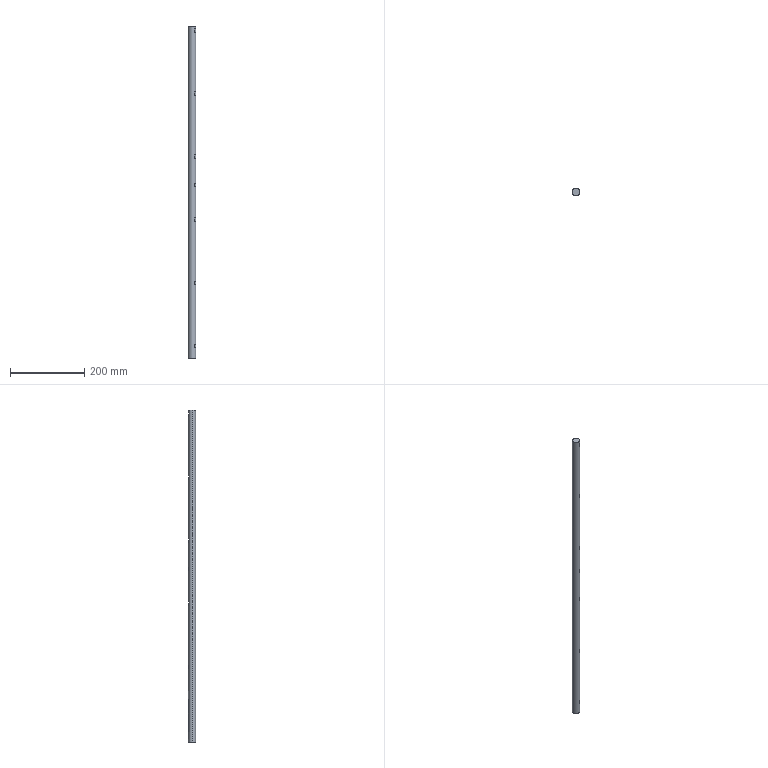Part | SolidWorks | features BaseBody 1 | 1 solid | 46 faces | box 20 x 20 x 895 mm | volume 280350 mm3 | plane 44 | cylinder 2 | commonest cylinder face diameters 20 x2
STEP:
#1=CARTESIAN_POINT('',(4.359,9.,877.5));
#2=VERTEX_POINT('',#1);
#3=CARTESIAN_POINT('',(-4.359,9.,877.5));
#4=VERTEX_POINT('',#3);
#5=CARTESIAN_POINT('',(0.,0.,877.5));
#6=DIRECTION('',(0.,0.,1.));
#7=DIRECTION('',(1.,0.,0.));
#8=AXIS2_PLACEMENT_3D('',#5,#6,#7);
#9=CIRCLE('',#8,10.);
#10=EDGE_CURVE('',#2,#4,#9,.T.);
#11=ORIENTED_EDGE('',*,*,#10,.F.);
#12=CARTESIAN_POINT('',(4.359,9.,887.5));
#13=VERTEX_POINT('',#12);
#14=CARTESIAN_POINT('',(4.359,9.,895.));
#15=DIRECTION('',(0.,0.,1.));
#16=VECTOR('',#15,1000.);
#17=LINE('',#14,#16);
#18=EDGE_CURVE('',#2,#13,#17,.T.);
#19=ORIENTED_EDGE('',*,*,#18,.T.);
#20=CARTESIAN_POINT('',(-4.359,9.,887.5));
#21=VERTEX_POINT('',#20);
#22=CARTESIAN_POINT('',(0.,0.,887.5));
#23=DIRECTION('',(0.,0.,1.));
#24=DIRECTION('',(1.,0.,0.));
#25=AXIS2_PLACEMENT_3D('',#22,#23,#24);
#26=CIRCLE('',#25,10.);
#27=EDGE_CURVE('',#13,#21,#26,.T.);
#28=ORIENTED_EDGE('',*,*,#27,.T.);
#29=CARTESIAN_POINT('',(-4.359,9.,895.));
#30=DIRECTION('',(0.,0.,-1.));
#31=VECTOR('',#30,1000.);
#32=LINE('',#29,#31);
#33=EDGE_CURVE('',#21,#4,#32,.T.);
#34=ORIENTED_EDGE('',*,*,#33,.T.);
#35=EDGE_LOOP('',(#11,#19,#28,#34));
#36=FACE_BOUND('',#35,.T.);
#37=CARTESIAN_POINT('',(4.359,9.,707.5));
#38=VERTEX_POINT('',#37);
#39=CARTESIAN_POINT('',(-4.359,9.,707.5));
#40=VERTEX_POINT('',#39);
#41=CARTESIAN_POINT('',(0.,0.,707.5));
#42=DIRECTION('',(0.,0.,1.));
#43=DIRECTION('',(1.,0.,0.));
#44=AXIS2_PLACEMENT_3D('',#41,#42,#43);
#45=CIRCLE('',#44,10.);
#46=EDGE_CURVE('',#38,#40,#45,.T.);
#47=ORIENTED_EDGE('',*,*,#46,.F.);
#48=CARTESIAN_POINT('',(4.359,9.,717.5));
#49=VERTEX_POINT('',#48);
#50=CARTESIAN_POINT('',(4.359,9.,895.));
#51=DIRECTION('',(0.,0.,1.));
#52=VECTOR('',#51,1000.);
#53=LINE('',#50,#52);
#54=EDGE_CURVE('',#38,#49,#53,.T.);
#55=ORIENTED_EDGE('',*,*,#54,.T.);
#56=CARTESIAN_POINT('',(-4.359,9.,717.5));
#57=VERTEX_POINT('',#56);
#58=CARTESIAN_POINT('',(0.,0.,717.5));
#59=DIRECTION('',(0.,0.,1.));
#60=DIRECTION('',(1.,0.,0.));
#61=AXIS2_PLACEMENT_3D('',#58,#59,#60);
#62=CIRCLE('',#61,10.);
#63=EDGE_CURVE('',#49,#57,#62,.T.);
#64=ORIENTED_EDGE('',*,*,#63,.T.);
#65=CARTESIAN_POINT('',(-4.359,9.,895.));
#66=DIRECTION('',(0.,0.,-1.));
#67=VECTOR('',#66,1000.);
#68=LINE('',#65,#67);
#69=EDGE_CURVE('',#57,#40,#68,.T.);
#70=ORIENTED_EDGE('',*,*,#69,.T.);
#71=EDGE_LOOP('',(#47,#55,#64,#70));
#72=FACE_BOUND('',#71,.T.);
#73=CARTESIAN_POINT('',(4.359,9.,537.5));
#74=VERTEX_POINT('',#73);
#75=CARTESIAN_POINT('',(-4.359,9.,537.5));
#76=VERTEX_POINT('',#75);
#77=CARTESIAN_POINT('',(0.,0.,537.5));
#78=DIRECTION('',(0.,0.,1.));
#79=DIRECTION('',(1.,0.,0.));
#80=AXIS2_PLACEMENT_3D('',#77,#78,#79);
#81=CIRCLE('',#80,10.);
#82=EDGE_CURVE('',#74,#76,#81,.T.);
#83=ORIENTED_EDGE('',*,*,#82,.F.);
#84=CARTESIAN_POINT('',(4.359,9.,547.5));
#85=VERTEX_POINT('',#84);
#86=CARTESIAN_POINT('',(4.359,9.,895.));
#87=DIRECTION('',(0.,0.,1.));
#88=VECTOR('',#87,1000.);
#89=LINE('',#86,#88);
#90=EDGE_CURVE('',#74,#85,#89,.T.);
#91=ORIENTED_EDGE('',*,*,#90,.T.);
#92=CARTESIAN_POINT('',(-4.359,9.,547.5));
#93=VERTEX_POINT('',#92);
#94=CARTESIAN_POINT('',(0.,0.,547.5));
#95=DIRECTION('',(0.,0.,1.));
#96=DIRECTION('',(1.,0.,0.));
#97=AXIS2_PLACEMENT_3D('',#94,#95,#96);
#98=CIRCLE('',#97,10.);
#99=EDGE_CURVE('',#85,#93,#98,.T.);
#100=ORIENTED_EDGE('',*,*,#99,.T.);
#101=CARTESIAN_POINT('',(-4.359,9.,895.));
#102=DIRECTION('',(0.,0.,-1.));
#103=VECTOR('',#102,1000.);
#104=LINE('',#101,#103);
#105=EDGE_CURVE('',#93,#76,#104,.T.);
#106=ORIENTED_EDGE('',*,*,#105,.T.);
#107=EDGE_LOOP('',(#83,#91,#100,#106));
#108=FACE_BOUND('',#107,.T.);
#109=CARTESIAN_POINT('',(4.359,9.,367.5));
#110=VERTEX_POINT('',#109);
#111=CARTESIAN_POINT('',(-4.359,9.,367.5));
#112=VERTEX_POINT('',#111);
#113=CARTESIAN_POINT('',(0.,0.,367.5));
#114=DIRECTION('',(0.,0.,1.));
#115=DIRECTION('',(1.,0.,0.));
#116=AXIS2_PLACEMENT_3D('',#113,#114,#115);
#117=CIRCLE('',#116,10.);
#118=EDGE_CURVE('',#110,#112,#117,.T.);
#119=ORIENTED_EDGE('',*,*,#118,.F.);
#120=CARTESIAN_POINT('',(4.359,9.,377.5));
#121=VERTEX_POINT('',#120);
#122=CARTESIAN_POINT('',(4.359,9.,895.));
#123=DIRECTION('',(0.,0.,1.));
#124=VECTOR('',#123,1000.);
#125=LINE('',#122,#124);
#126=EDGE_CURVE('',#110,#121,#125,.T.);
#127=ORIENTED_EDGE('',*,*,#126,.T.);
#128=CARTESIAN_POINT('',(-4.359,9.,377.5));
#129=VERTEX_POINT('',#128);
#130=CARTESIAN_POINT('',(0.,0.,377.5));
#131=DIRECTION('',(0.,0.,1.));
#132=DIRECTION('',(1.,0.,0.));
#133=AXIS2_PLACEMENT_3D('',#130,#131,#132);
#134=CIRCLE('',#133,10.);
#135=EDGE_CURVE('',#121,#129,#134,.T.);
#136=ORIENTED_EDGE('',*,*,#135,.T.);
#137=CARTESIAN_POINT('',(-4.359,9.,895.));
#138=DIRECTION('',(0.,0.,-1.));
#139=VECTOR('',#138,1000.);
#140=LINE('',#137,#139);
#141=EDGE_CURVE('',#129,#112,#140,.T.);
#142=ORIENTED_EDGE('',*,*,#141,.T.);
#143=EDGE_LOOP('',(#119,#127,#136,#142));
#144=FACE_BOUND('',#143,.T.);
#145=CARTESIAN_POINT('',(4.359,9.,197.5));
#146=VERTEX_POINT('',#145);
#147=CARTESIAN_POINT('',(-4.359,9.,197.5));
#148=VERTEX_POINT('',#147);
#149=CARTESIAN_POINT('',(0.,0.,197.5));
#150=DIRECTION('',(0.,0.,1.));
#151=DIRECTION('',(1.,0.,0.));
#152=AXIS2_PLACEMENT_3D('',#149,#150,#151);
#153=CIRCLE('',#152,10.);
#154=EDGE_CURVE('',#146,#148,#153,.T.);
#155=ORIENTED_EDGE('',*,*,#154,.F.);
#156=CARTESIAN_POINT('',(4.359,9.,207.5));
#157=VERTEX_POINT('',#156);
#158=CARTESIAN_POINT('',(4.359,9.,895.));
#159=DIRECTION('',(0.,0.,1.));
#160=VECTOR('',#159,1000.);
#161=LINE('',#158,#160);
#162=EDGE_CURVE('',#146,#157,#161,.T.);
#163=ORIENTED_EDGE('',*,*,#162,.T.);
#164=CARTESIAN_POINT('',(-4.359,9.,207.5));
#165=VERTEX_POINT('',#164);
#166=CARTESIAN_POINT('',(0.,0.,207.5));
#167=DIRECTION('',(0.,0.,1.));
#168=DIRECTION('',(1.,0.,0.));
#169=AXIS2_PLACEMENT_3D('',#166,#167,#168);
#170=CIRCLE('',#169,10.);
#171=EDGE_CURVE('',#157,#165,#170,.T.);
#172=ORIENTED_EDGE('',*,*,#171,.T.);
#173=CARTESIAN_POINT('',(-4.359,9.,895.));
#174=DIRECTION('',(0.,0.,-1.));
#175=VECTOR('',#174,1000.);
#176=LINE('',#173,#175);
#177=EDGE_CURVE('',#165,#148,#176,.T.);
#178=ORIENTED_EDGE('',*,*,#177,.T.);
#179=EDGE_LOOP('',(#155,#163,#172,#178));
#180=FACE_BOUND('',#179,.T.);
#181=CARTESIAN_POINT('',(4.359,9.,27.5));
#182=VERTEX_POINT('',#181);
#183=CARTESIAN_POINT('',(-4.359,9.,27.5));
#184=VERTEX_POINT('',#183);
#185=CARTESIAN_POINT('',(0.,0.,27.5));
#186=DIRECTION('',(0.,0.,1.));
#187=DIRECTION('',(1.,0.,0.));
#188=AXIS2_PLACEMENT_3D('',#185,#186,#187);
#189=CIRCLE('',#188,10.);
#190=EDGE_CURVE('',#182,#184,#189,.T.);
#191=ORIENTED_EDGE('',*,*,#190,.F.);
#192=CARTESIAN_POINT('',(4.359,9.,37.5));
#193=VERTEX_POINT('',#192);
#194=CARTESIAN_POINT('',(4.359,9.,895.));
#195=DIRECTION('',(0.,0.,1.));
#196=VECTOR('',#195,1000.);
#197=LINE('',#194,#196);
#198=EDGE_CURVE('',#182,#193,#197,.T.);
#199=ORIENTED_EDGE('',*,*,#198,.T.);
#200=CARTESIAN_POINT('',(-4.359,9.,37.5));
#201=VERTEX_POINT('',#200);
#202=CARTESIAN_POINT('',(0.,0.,37.5));
#203=DIRECTION('',(0.,0.,1.));
#204=DIRECTION('',(1.,0.,0.));
#205=AXIS2_PLACEMENT_3D('',#202,#203,#204);
#206=CIRCLE('',#205,10.);
#207=EDGE_CURVE('',#193,#201,#206,.T.);
#208=ORIENTED_EDGE('',*,*,#207,.T.);
#209=CARTESIAN_POINT('',(-4.359,9.,895.));
#210=DIRECTION('',(0.,0.,-1.));
#211=VECTOR('',#210,1000.);
#212=LINE('',#209,#211);
#213=EDGE_CURVE('',#201,#184,#212,.T.);
#214=ORIENTED_EDGE('',*,*,#213,.T.);
#215=EDGE_LOOP('',(#191,#199,#208,#214));
#216=FACE_BOUND('',#215,.T.);
#217=CARTESIAN_POINT('',(4.359,9.,461.5));
#218=VERTEX_POINT('',#217);
#219=CARTESIAN_POINT('',(-4.359,9.,461.5));
#220=VERTEX_POINT('',#219);
#221=CARTESIAN_POINT('',(0.,0.,461.5));
#222=DIRECTION('',(0.,0.,1.));
#223=DIRECTION('',(1.,0.,0.));
#224=AXIS2_PLACEMENT_3D('',#221,#222,#223);
#225=CIRCLE('',#224,10.);
#226=EDGE_CURVE('',#218,#220,#225,.T.);
#227=ORIENTED_EDGE('',*,*,#226,.F.);
#228=CARTESIAN_POINT('',(4.359,9.,471.5));
#229=VERTEX_POINT('',#228);
#230=CARTESIAN_POINT('',(4.359,9.,461.5));
#231=DIRECTION('',(0.,0.,1.));
#232=VECTOR('',#231,1000.);
#233=LINE('',#230,#232);
#234=EDGE_CURVE('',#218,#229,#233,.T.);
#235=ORIENTED_EDGE('',*,*,#234,.T.);
#236=CARTESIAN_POINT('',(-4.359,9.,471.5));
#237=VERTEX_POINT('',#236);
#238=CARTESIAN_POINT('',(0.,0.,471.5));
#239=DIRECTION('',(0.,0.,1.));
#240=DIRECTION('',(1.,0.,0.));
#241=AXIS2_PLACEMENT_3D('',#238,#239,#240);
#242=CIRCLE('',#241,10.);
#243=EDGE_CURVE('',#229,#237,#242,.T.);
#244=ORIENTED_EDGE('',*,*,#243,.T.);
#245=CARTESIAN_POINT('',(-4.359,9.,461.5));
#246=DIRECTION('',(0.,0.,1.));
#247=VECTOR('',#246,1000.);
#248=LINE('',#245,#247);
#249=EDGE_CURVE('',#220,#237,#248,.T.);
#250=ORIENTED_EDGE('',*,*,#249,.F.);
#251=EDGE_LOOP('',(#227,#235,#244,#250));
#252=FACE_BOUND('',#251,.T.);
#253=CARTESIAN_POINT('',(10.,0.,895.));
#254=VERTEX_POINT('',#253);
#255=CARTESIAN_POINT('',(-10.,0.,895.));
#256=VERTEX_POINT('',#255);
#257=CARTESIAN_POINT('',(0.,0.,895.));
#258=DIRECTION('',(0.,0.,1.));
#259=DIRECTION('',(1.,0.,0.));
#260=AXIS2_PLACEMENT_3D('',#257,#258,#259);
#261=CIRCLE('',#260,10.);
#262=EDGE_CURVE('',#254,#256,#261,.T.);
#263=ORIENTED_EDGE('',*,*,#262,.F.);
#264=CARTESIAN_POINT('',(10.,0.,0.));
#265=VERTEX_POINT('',#264);
#266=CARTESIAN_POINT('',(10.,0.,895.));
#267=DIRECTION('',(0.,0.,-1.));
#268=VECTOR('',#267,1000.);
#269=LINE('',#266,#268);
#270=EDGE_CURVE('',#254,#265,#269,.T.);
#271=ORIENTED_EDGE('',*,*,#270,.T.);
#272=CARTESIAN_POINT('',(-10.,0.,0.));
#273=VERTEX_POINT('',#272);
#274=CARTESIAN_POINT('',(0.,0.,0.));
#275=DIRECTION('',(0.,0.,1.));
#276=DIRECTION('',(1.,0.,0.));
#277=AXIS2_PLACEMENT_3D('',#274,#275,#276);
#278=CIRCLE('',#277,10.);
#279=EDGE_CURVE('',#265,#273,#278,.T.);
#280=ORIENTED_EDGE('',*,*,#279,.T.);
#281=CARTESIAN_POINT('',(-10.,0.,895.));
#282=DIRECTION('',(0.,0.,-1.));
#283=VECTOR('',#282,1000.);
#284=LINE('',#281,#283);
#285=EDGE_CURVE('',#256,#273,#284,.T.);
#286=ORIENTED_EDGE('',*,*,#285,.F.);
#287=EDGE_LOOP('',(#263,#271,#280,#286));
#288=FACE_OUTER_BOUND('',#287,.T.);
#289=CARTESIAN_POINT('',(0.,0.,895.));
#290=DIRECTION('',(0.,0.,-1.));
#291=DIRECTION('',(-1.,0.,0.));
#292=AXIS2_PLACEMENT_3D('',#289,#290,#291);
#293=CYLINDRICAL_SURFACE('',#292,10.);
#294=ADVANCED_FACE('',(#36,#72,#108,#144,#180,#216,#252,#288),#293,.T.);
#295=CARTESIAN_POINT('',(5.615,-8.275,471.5));
#296=VERTEX_POINT('',#295);
#297=CARTESIAN_POINT('',(9.974,-0.7251,471.5));
#298=VERTEX_POINT('',#297);
#299=CARTESIAN_POINT('',(0.,0.,471.5));
#300=DIRECTION('',(0.,0.,1.));
#301=DIRECTION('',(1.,0.,0.));
#302=AXIS2_PLACEMENT_3D('',#299,#300,#301);
#303=CIRCLE('',#302,10.);
#304=EDGE_CURVE('',#296,#298,#303,.T.);
#305=ORIENTED_EDGE('',*,*,#304,.F.);
#306=CARTESIAN_POINT('',(9.974,-0.7251,471.5));
#307=DIRECTION('',(-0.5,-0.866,0.));
#308=VECTOR('',#307,1000.);
#309=LINE('',#306,#308);
#310=EDGE_CURVE('',#298,#296,#309,.T.);
#311=ORIENTED_EDGE('',*,*,#310,.F.);
#312=EDGE_LOOP('',(#305,#311));
#313=FACE_OUTER_BOUND('',#312,.T.);
#314=CARTESIAN_POINT('',(0.,0.,471.5));
#315=DIRECTION('',(0.,0.,1.));
#316=DIRECTION('',(1.,0.,0.));
#317=AXIS2_PLACEMENT_3D('',#314,#315,#316);
#318=PLANE('',#317);
#319=ADVANCED_FACE('',(#313),#318,.F.);
#320=CARTESIAN_POINT('',(5.615,-8.275,461.5));
#321=VERTEX_POINT('',#320);
#322=CARTESIAN_POINT('',(9.974,-0.7251,461.5));
#323=VERTEX_POINT('',#322);
#324=CARTESIAN_POINT('',(0.,0.,461.5));
#325=DIRECTION('',(0.,0.,1.));
#326=DIRECTION('',(1.,0.,0.));
#327=AXIS2_PLACEMENT_3D('',#324,#325,#326);
#328=CIRCLE('',#327,10.);
#329=EDGE_CURVE('',#321,#323,#328,.T.);
#330=ORIENTED_EDGE('',*,*,#329,.T.);
#331=CARTESIAN_POINT('',(9.974,-0.7251,461.5));
#332=DIRECTION('',(-0.5,-0.866,0.));
#333=VECTOR('',#332,1000.);
#334=LINE('',#331,#333);
#335=EDGE_CURVE('',#323,#321,#334,.T.);
#336=ORIENTED_EDGE('',*,*,#335,.T.);
#337=EDGE_LOOP('',(#330,#336));
#338=FACE_OUTER_BOUND('',#337,.T.);
#339=CARTESIAN_POINT('',(0.,0.,461.5));
#340=DIRECTION('',(0.,0.,1.));
#341=DIRECTION('',(1.,0.,0.));
#342=AXIS2_PLACEMENT_3D('',#339,#340,#341);
#343=PLANE('',#342);
#344=ADVANCED_FACE('',(#338),#343,.T.);
#345=ORIENTED_EDGE('',*,*,#310,.T.);
#346=CARTESIAN_POINT('',(5.615,-8.275,461.5));
#347=DIRECTION('',(0.,0.,1.));
#348=VECTOR('',#347,1000.);
#349=LINE('',#346,#348);
#350=EDGE_CURVE('',#321,#296,#349,.T.);
#351=ORIENTED_EDGE('',*,*,#350,.F.);
#352=ORIENTED_EDGE('',*,*,#335,.F.);
#353=CARTESIAN_POINT('',(9.974,-0.7251,461.5));
#354=DIRECTION('',(0.,0.,1.));
#355=VECTOR('',#354,1000.);
#356=LINE('',#353,#355);
#357=EDGE_CURVE('',#323,#298,#356,.T.);
#358=ORIENTED_EDGE('',*,*,#357,.T.);
#359=EDGE_LOOP('',(#345,#351,#352,#358));
#360=FACE_OUTER_BOUND('',#359,.T.);
#361=CARTESIAN_POINT('',(9.974,-0.7251,461.5));
#362=DIRECTION('',(-0.866,0.5,0.));
#363=DIRECTION('',(0.,0.,1.));
#364=AXIS2_PLACEMENT_3D('',#361,#362,#363);
#365=PLANE('',#364);
#366=ADVANCED_FACE('',(#360),#365,.F.);
#367=ORIENTED_EDGE('',*,*,#243,.F.);
#368=CARTESIAN_POINT('',(-4.359,9.,471.5));
#369=DIRECTION('',(1.,0.,0.));
#370=VECTOR('',#369,1000.);
#371=LINE('',#368,#370);
#372=EDGE_CURVE('',#237,#229,#371,.T.);
#373=ORIENTED_EDGE('',*,*,#372,.F.);
#374=EDGE_LOOP('',(#367,#373));
#375=FACE_OUTER_BOUND('',#374,.T.);
#376=CARTESIAN_POINT('',(0.,0.,471.5));
#377=DIRECTION('',(0.,0.,1.));
#378=DIRECTION('',(1.,0.,0.));
#379=AXIS2_PLACEMENT_3D('',#376,#377,#378);
#380=PLANE('',#379);
#381=ADVANCED_FACE('',(#375),#380,.F.);
#382=ORIENTED_EDGE('',*,*,#226,.T.);
#383=CARTESIAN_POINT('',(-4.359,9.,461.5));
#384=DIRECTION('',(1.,0.,0.));
#385=VECTOR('',#384,1000.);
#386=LINE('',#383,#385);
#387=EDGE_CURVE('',#220,#218,#386,.T.);
#388=ORIENTED_EDGE('',*,*,#387,.T.);
#389=EDGE_LOOP('',(#382,#388));
#390=FACE_OUTER_BOUND('',#389,.T.);
#391=CARTESIAN_POINT('',(0.,0.,461.5));
#392=DIRECTION('',(0.,0.,1.));
#393=DIRECTION('',(1.,0.,0.));
#394=AXIS2_PLACEMENT_3D('',#391,#392,#393);
#395=PLANE('',#394);
#396=ADVANCED_FACE('',(#390),#395,.T.);
#397=ORIENTED_EDGE('',*,*,#372,.T.);
#398=ORIENTED_EDGE('',*,*,#234,.F.);
#399=ORIENTED_EDGE('',*,*,#387,.F.);
#400=ORIENTED_EDGE('',*,*,#249,.T.);
#401=EDGE_LOOP('',(#397,#398,#399,#400));
#402=FACE_OUTER_BOUND('',#401,.T.);
#403=CARTESIAN_POINT('',(-4.359,9.,461.5));
#404=DIRECTION('',(0.,-1.,0.));
#405=DIRECTION('',(0.,0.,-1.));
#406=AXIS2_PLACEMENT_3D('',#403,#404,#405);
#407=PLANE('',#406);
#408=ADVANCED_FACE('',(#402),#407,.F.);
#409=CARTESIAN_POINT('',(9.974,-0.7251,37.5));
#410=VERTEX_POINT('',#409);
#411=CARTESIAN_POINT('',(5.615,-8.275,37.5));
#412=VERTEX_POINT('',#411);
#413=CARTESIAN_POINT('',(13.76,5.834,37.5));
#414=DIRECTION('',(-0.5,-0.866,0.));
#415=VECTOR('',#414,1000.);
#416=LINE('',#413,#415);
#417=EDGE_CURVE('',#410,#412,#416,.T.);
#418=ORIENTED_EDGE('',*,*,#417,.F.);
#419=CARTESIAN_POINT('',(0.,0.,37.5));
#420=DIRECTION('',(0.,0.,1.));
#421=DIRECTION('',(1.,0.,0.));
#422=AXIS2_PLACEMENT_3D('',#419,#420,#421);
#423=CIRCLE('',#422,10.);
#424=EDGE_CURVE('',#412,#410,#423,.T.);
#425=ORIENTED_EDGE('',*,*,#424,.F.);
#426=EDGE_LOOP('',(#418,#425));
#427=FACE_OUTER_BOUND('',#426,.T.);
#428=CARTESIAN_POINT('',(0.,0.,37.5));
#429=DIRECTION('',(0.,0.,1.));
#430=DIRECTION('',(1.,0.,0.));
#431=AXIS2_PLACEMENT_3D('',#428,#429,#430);
#432=PLANE('',#431);
#433=ADVANCED_FACE('',(#427),#432,.F.);
#434=CARTESIAN_POINT('',(5.615,-8.275,27.5));
#435=VERTEX_POINT('',#434);
#436=CARTESIAN_POINT('',(9.974,-0.7251,27.5));
#437=VERTEX_POINT('',#436);
#438=CARTESIAN_POINT('',(0.,0.,27.5));
#439=DIRECTION('',(0.,0.,1.));
#440=DIRECTION('',(1.,0.,0.));
#441=AXIS2_PLACEMENT_3D('',#438,#439,#440);
#442=CIRCLE('',#441,10.);
#443=EDGE_CURVE('',#435,#437,#442,.T.);
#444=ORIENTED_EDGE('',*,*,#443,.T.);
#445=CARTESIAN_POINT('',(13.76,5.834,27.5));
#446=DIRECTION('',(-0.5,-0.866,0.));
#447=VECTOR('',#446,1000.);
#448=LINE('',#445,#447);
#449=EDGE_CURVE('',#437,#435,#448,.T.);
#450=ORIENTED_EDGE('',*,*,#449,.T.);
#451=EDGE_LOOP('',(#444,#450));
#452=FACE_OUTER_BOUND('',#451,.T.);
#453=CARTESIAN_POINT('',(0.,0.,27.5));
#454=DIRECTION('',(0.,0.,1.));
#455=DIRECTION('',(1.,0.,0.));
#456=AXIS2_PLACEMENT_3D('',#453,#454,#455);
#457=PLANE('',#456);
#458=ADVANCED_FACE('',(#452),#457,.T.);
#459=ORIENTED_EDGE('',*,*,#417,.T.);
#460=CARTESIAN_POINT('',(5.615,-8.275,895.));
#461=DIRECTION('',(0.,0.,1.));
#462=VECTOR('',#461,1000.);
#463=LINE('',#460,#462);
#464=EDGE_CURVE('',#435,#412,#463,.T.);
#465=ORIENTED_EDGE('',*,*,#464,.F.);
#466=ORIENTED_EDGE('',*,*,#449,.F.);
#467=CARTESIAN_POINT('',(9.974,-0.7251,895.));
#468=DIRECTION('',(0.,0.,-1.));
#469=VECTOR('',#468,1000.);
#470=LINE('',#467,#469);
#471=EDGE_CURVE('',#410,#437,#470,.T.);
#472=ORIENTED_EDGE('',*,*,#471,.F.);
#473=EDGE_LOOP('',(#459,#465,#466,#472));
#474=FACE_OUTER_BOUND('',#473,.T.);
#475=CARTESIAN_POINT('',(13.76,5.834,27.5));
#476=DIRECTION('',(-0.866,0.5,0.));
#477=DIRECTION('',(0.,0.,1.));
#478=AXIS2_PLACEMENT_3D('',#475,#476,#477);
#479=PLANE('',#478);
#480=ADVANCED_FACE('',(#474),#479,.F.);
#481=CARTESIAN_POINT('',(-8.178,9.,37.5));
#482=DIRECTION('',(1.,0.,0.));
#483=VECTOR('',#482,1000.);
#484=LINE('',#481,#483);
#485=EDGE_CURVE('',#201,#193,#484,.T.);
#486=ORIENTED_EDGE('',*,*,#485,.F.);
#487=ORIENTED_EDGE('',*,*,#207,.F.);
#488=EDGE_LOOP('',(#486,#487));
#489=FACE_OUTER_BOUND('',#488,.T.);
#490=CARTESIAN_POINT('',(0.,0.,37.5));
#491=DIRECTION('',(0.,0.,1.));
#492=DIRECTION('',(1.,0.,0.));
#493=AXIS2_PLACEMENT_3D('',#490,#491,#492);
#494=PLANE('',#493);
#495=ADVANCED_FACE('',(#489),#494,.F.);
#496=ORIENTED_EDGE('',*,*,#190,.T.);
#497=CARTESIAN_POINT('',(-8.178,9.,27.5));
#498=DIRECTION('',(1.,0.,0.));
#499=VECTOR('',#498,1000.);
#500=LINE('',#497,#499);
#501=EDGE_CURVE('',#184,#182,#500,.T.);
#502=ORIENTED_EDGE('',*,*,#501,.T.);
#503=EDGE_LOOP('',(#496,#502));
#504=FACE_OUTER_BOUND('',#503,.T.);
#505=CARTESIAN_POINT('',(0.,0.,27.5));
#506=DIRECTION('',(0.,0.,1.));
#507=DIRECTION('',(1.,0.,0.));
#508=AXIS2_PLACEMENT_3D('',#505,#506,#507);
#509=PLANE('',#508);
#510=ADVANCED_FACE('',(#504),#509,.T.);
#511=ORIENTED_EDGE('',*,*,#485,.T.);
#512=ORIENTED_EDGE('',*,*,#198,.F.);
#513=ORIENTED_EDGE('',*,*,#501,.F.);
#514=ORIENTED_EDGE('',*,*,#213,.F.);
#515=EDGE_LOOP('',(#511,#512,#513,#514));
#516=FACE_OUTER_BOUND('',#515,.T.);
#517=CARTESIAN_POINT('',(-8.178,9.,27.5));
#518=DIRECTION('',(0.,-1.,0.));
#519=DIRECTION('',(0.,0.,-1.));
#520=AXIS2_PLACEMENT_3D('',#517,#518,#519);
#521=PLANE('',#520);
#522=ADVANCED_FACE('',(#516),#521,.F.);
#523=CARTESIAN_POINT('',(9.974,-0.7251,207.5));
#524=VERTEX_POINT('',#523);
#525=CARTESIAN_POINT('',(5.615,-8.275,207.5));
#526=VERTEX_POINT('',#525);
#527=CARTESIAN_POINT('',(13.76,5.834,207.5));
#528=DIRECTION('',(-0.5,-0.866,0.));
#529=VECTOR('',#528,1000.);
#530=LINE('',#527,#529);
#531=EDGE_CURVE('',#524,#526,#530,.T.);
#532=ORIENTED_EDGE('',*,*,#531,.F.);
#533=CARTESIAN_POINT('',(0.,0.,207.5));
#534=DIRECTION('',(0.,0.,1.));
#535=DIRECTION('',(1.,0.,0.));
#536=AXIS2_PLACEMENT_3D('',#533,#534,#535);
#537=CIRCLE('',#536,10.);
#538=EDGE_CURVE('',#526,#524,#537,.T.);
#539=ORIENTED_EDGE('',*,*,#538,.F.);
#540=EDGE_LOOP('',(#532,#539));
#541=FACE_OUTER_BOUND('',#540,.T.);
#542=CARTESIAN_POINT('',(0.,0.,207.5));
#543=DIRECTION('',(0.,0.,1.));
#544=DIRECTION('',(1.,0.,0.));
#545=AXIS2_PLACEMENT_3D('',#542,#543,#544);
#546=PLANE('',#545);
#547=ADVANCED_FACE('',(#541),#546,.F.);
#548=CARTESIAN_POINT('',(5.615,-8.275,197.5));
#549=VERTEX_POINT('',#548);
#550=CARTESIAN_POINT('',(9.974,-0.7251,197.5));
#551=VERTEX_POINT('',#550);
#552=CARTESIAN_POINT('',(0.,0.,197.5));
#553=DIRECTION('',(0.,0.,1.));
#554=DIRECTION('',(1.,0.,0.));
#555=AXIS2_PLACEMENT_3D('',#552,#553,#554);
#556=CIRCLE('',#555,10.);
#557=EDGE_CURVE('',#549,#551,#556,.T.);
#558=ORIENTED_EDGE('',*,*,#557,.T.);
#559=CARTESIAN_POINT('',(13.76,5.834,197.5));
#560=DIRECTION('',(-0.5,-0.866,0.));
#561=VECTOR('',#560,1000.);
#562=LINE('',#559,#561);
#563=EDGE_CURVE('',#551,#549,#562,.T.);
#564=ORIENTED_EDGE('',*,*,#563,.T.);
#565=EDGE_LOOP('',(#558,#564));
#566=FACE_OUTER_BOUND('',#565,.T.);
#567=CARTESIAN_POINT('',(0.,0.,197.5));
#568=DIRECTION('',(0.,0.,1.));
#569=DIRECTION('',(1.,0.,0.));
#570=AXIS2_PLACEMENT_3D('',#567,#568,#569);
#571=PLANE('',#570);
#572=ADVANCED_FACE('',(#566),#571,.T.);
#573=ORIENTED_EDGE('',*,*,#531,.T.);
#574=CARTESIAN_POINT('',(5.615,-8.275,895.));
#575=DIRECTION('',(0.,0.,1.));
#576=VECTOR('',#575,1000.);
#577=LINE('',#574,#576);
#578=EDGE_CURVE('',#549,#526,#577,.T.);
#579=ORIENTED_EDGE('',*,*,#578,.F.);
#580=ORIENTED_EDGE('',*,*,#563,.F.);
#581=CARTESIAN_POINT('',(9.974,-0.7251,895.));
#582=DIRECTION('',(0.,0.,-1.));
#583=VECTOR('',#582,1000.);
#584=LINE('',#581,#583);
#585=EDGE_CURVE('',#524,#551,#584,.T.);
#586=ORIENTED_EDGE('',*,*,#585,.F.);
#587=EDGE_LOOP('',(#573,#579,#580,#586));
#588=FACE_OUTER_BOUND('',#587,.T.);
#589=CARTESIAN_POINT('',(13.76,5.834,197.5));
#590=DIRECTION('',(-0.866,0.5,0.));
#591=DIRECTION('',(0.,0.,1.));
#592=AXIS2_PLACEMENT_3D('',#589,#590,#591);
#593=PLANE('',#592);
#594=ADVANCED_FACE('',(#588),#593,.F.);
#595=CARTESIAN_POINT('',(-8.178,9.,207.5));
#596=DIRECTION('',(1.,0.,0.));
#597=VECTOR('',#596,1000.);
#598=LINE('',#595,#597);
#599=EDGE_CURVE('',#165,#157,#598,.T.);
#600=ORIENTED_EDGE('',*,*,#599,.F.);
#601=ORIENTED_EDGE('',*,*,#171,.F.);
#602=EDGE_LOOP('',(#600,#601));
#603=FACE_OUTER_BOUND('',#602,.T.);
#604=CARTESIAN_POINT('',(0.,0.,207.5));
#605=DIRECTION('',(0.,0.,1.));
#606=DIRECTION('',(1.,0.,0.));
#607=AXIS2_PLACEMENT_3D('',#604,#605,#606);
#608=PLANE('',#607);
#609=ADVANCED_FACE('',(#603),#608,.F.);
#610=ORIENTED_EDGE('',*,*,#154,.T.);
#611=CARTESIAN_POINT('',(-8.178,9.,197.5));
#612=DIRECTION('',(1.,0.,0.));
#613=VECTOR('',#612,1000.);
#614=LINE('',#611,#613);
#615=EDGE_CURVE('',#148,#146,#614,.T.);
#616=ORIENTED_EDGE('',*,*,#615,.T.);
#617=EDGE_LOOP('',(#610,#616));
#618=FACE_OUTER_BOUND('',#617,.T.);
#619=CARTESIAN_POINT('',(0.,0.,197.5));
#620=DIRECTION('',(0.,0.,1.));
#621=DIRECTION('',(1.,0.,0.));
#622=AXIS2_PLACEMENT_3D('',#619,#620,#621);
#623=PLANE('',#622);
#624=ADVANCED_FACE('',(#618),#623,.T.);
#625=ORIENTED_EDGE('',*,*,#599,.T.);
#626=ORIENTED_EDGE('',*,*,#162,.F.);
#627=ORIENTED_EDGE('',*,*,#615,.F.);
#628=ORIENTED_EDGE('',*,*,#177,.F.);
#629=EDGE_LOOP('',(#625,#626,#627,#628));
#630=FACE_OUTER_BOUND('',#629,.T.);
#631=CARTESIAN_POINT('',(-8.178,9.,197.5));
#632=DIRECTION('',(0.,-1.,0.));
#633=DIRECTION('',(0.,0.,-1.));
#634=AXIS2_PLACEMENT_3D('',#631,#632,#633);
#635=PLANE('',#634);
#636=ADVANCED_FACE('',(#630),#635,.F.);
#637=CARTESIAN_POINT('',(9.974,-0.7251,377.5));
#638=VERTEX_POINT('',#637);
#639=CARTESIAN_POINT('',(5.615,-8.275,377.5));
#640=VERTEX_POINT('',#639);
#641=CARTESIAN_POINT('',(13.76,5.834,377.5));
#642=DIRECTION('',(-0.5,-0.866,0.));
#643=VECTOR('',#642,1000.);
#644=LINE('',#641,#643);
#645=EDGE_CURVE('',#638,#640,#644,.T.);
#646=ORIENTED_EDGE('',*,*,#645,.F.);
#647=CARTESIAN_POINT('',(0.,0.,377.5));
#648=DIRECTION('',(0.,0.,1.));
#649=DIRECTION('',(1.,0.,0.));
#650=AXIS2_PLACEMENT_3D('',#647,#648,#649);
#651=CIRCLE('',#650,10.);
#652=EDGE_CURVE('',#640,#638,#651,.T.);
#653=ORIENTED_EDGE('',*,*,#652,.F.);
#654=EDGE_LOOP('',(#646,#653));
#655=FACE_OUTER_BOUND('',#654,.T.);
#656=CARTESIAN_POINT('',(0.,0.,377.5));
#657=DIRECTION('',(0.,0.,1.));
#658=DIRECTION('',(1.,0.,0.));
#659=AXIS2_PLACEMENT_3D('',#656,#657,#658);
#660=PLANE('',#659);
#661=ADVANCED_FACE('',(#655),#660,.F.);
#662=CARTESIAN_POINT('',(5.615,-8.275,367.5));
#663=VERTEX_POINT('',#662);
#664=CARTESIAN_POINT('',(9.974,-0.7251,367.5));
#665=VERTEX_POINT('',#664);
#666=CARTESIAN_POINT('',(0.,0.,367.5));
#667=DIRECTION('',(0.,0.,1.));
#668=DIRECTION('',(1.,0.,0.));
#669=AXIS2_PLACEMENT_3D('',#666,#667,#668);
#670=CIRCLE('',#669,10.);
#671=EDGE_CURVE('',#663,#665,#670,.T.);
#672=ORIENTED_EDGE('',*,*,#671,.T.);
#673=CARTESIAN_POINT('',(13.76,5.834,367.5));
#674=DIRECTION('',(-0.5,-0.866,0.));
#675=VECTOR('',#674,1000.);
#676=LINE('',#673,#675);
#677=EDGE_CURVE('',#665,#663,#676,.T.);
#678=ORIENTED_EDGE('',*,*,#677,.T.);
#679=EDGE_LOOP('',(#672,#678));
#680=FACE_OUTER_BOUND('',#679,.T.);
#681=CARTESIAN_POINT('',(0.,0.,367.5));
#682=DIRECTION('',(0.,0.,1.));
#683=DIRECTION('',(1.,0.,0.));
#684=AXIS2_PLACEMENT_3D('',#681,#682,#683);
#685=PLANE('',#684);
#686=ADVANCED_FACE('',(#680),#685,.T.);
#687=ORIENTED_EDGE('',*,*,#645,.T.);
#688=CARTESIAN_POINT('',(5.615,-8.275,895.));
#689=DIRECTION('',(0.,0.,1.));
#690=VECTOR('',#689,1000.);
#691=LINE('',#688,#690);
#692=EDGE_CURVE('',#663,#640,#691,.T.);
#693=ORIENTED_EDGE('',*,*,#692,.F.);
#694=ORIENTED_EDGE('',*,*,#677,.F.);
#695=CARTESIAN_POINT('',(9.974,-0.7251,895.));
#696=DIRECTION('',(0.,0.,-1.));
#697=VECTOR('',#696,1000.);
#698=LINE('',#695,#697);
#699=EDGE_CURVE('',#638,#665,#698,.T.);
#700=ORIENTED_EDGE('',*,*,#699,.F.);
#701=EDGE_LOOP('',(#687,#693,#694,#700));
#702=FACE_OUTER_BOUND('',#701,.T.);
#703=CARTESIAN_POINT('',(13.76,5.834,367.5));
#704=DIRECTION('',(-0.866,0.5,0.));
#705=DIRECTION('',(0.,0.,1.));
#706=AXIS2_PLACEMENT_3D('',#703,#704,#705);
#707=PLANE('',#706);
#708=ADVANCED_FACE('',(#702),#707,.F.);
#709=CARTESIAN_POINT('',(-8.178,9.,377.5));
#710=DIRECTION('',(1.,0.,0.));
#711=VECTOR('',#710,1000.);
#712=LINE('',#709,#711);
#713=EDGE_CURVE('',#129,#121,#712,.T.);
#714=ORIENTED_EDGE('',*,*,#713,.F.);
#715=ORIENTED_EDGE('',*,*,#135,.F.);
#716=EDGE_LOOP('',(#714,#715));
#717=FACE_OUTER_BOUND('',#716,.T.);
#718=CARTESIAN_POINT('',(0.,0.,377.5));
#719=DIRECTION('',(0.,0.,1.));
#720=DIRECTION('',(1.,0.,0.));
#721=AXIS2_PLACEMENT_3D('',#718,#719,#720);
#722=PLANE('',#721);
#723=ADVANCED_FACE('',(#717),#722,.F.);
#724=ORIENTED_EDGE('',*,*,#118,.T.);
#725=CARTESIAN_POINT('',(-8.178,9.,367.5));
#726=DIRECTION('',(1.,0.,0.));
#727=VECTOR('',#726,1000.);
#728=LINE('',#725,#727);
#729=EDGE_CURVE('',#112,#110,#728,.T.);
#730=ORIENTED_EDGE('',*,*,#729,.T.);
#731=EDGE_LOOP('',(#724,#730));
#732=FACE_OUTER_BOUND('',#731,.T.);
#733=CARTESIAN_POINT('',(0.,0.,367.5));
#734=DIRECTION('',(0.,0.,1.));
#735=DIRECTION('',(1.,0.,0.));
#736=AXIS2_PLACEMENT_3D('',#733,#734,#735);
#737=PLANE('',#736);
#738=ADVANCED_FACE('',(#732),#737,.T.);
#739=ORIENTED_EDGE('',*,*,#713,.T.);
#740=ORIENTED_EDGE('',*,*,#126,.F.);
#741=ORIENTED_EDGE('',*,*,#729,.F.);
#742=ORIENTED_EDGE('',*,*,#141,.F.);
#743=EDGE_LOOP('',(#739,#740,#741,#742));
#744=FACE_OUTER_BOUND('',#743,.T.);
#745=CARTESIAN_POINT('',(-8.178,9.,367.5));
#746=DIRECTION('',(0.,-1.,0.));
#747=DIRECTION('',(0.,0.,-1.));
#748=AXIS2_PLACEMENT_3D('',#745,#746,#747);
#749=PLANE('',#748);
#750=ADVANCED_FACE('',(#744),#749,.F.);
#751=CARTESIAN_POINT('',(9.974,-0.7251,547.5));
#752=VERTEX_POINT('',#751);
#753=CARTESIAN_POINT('',(5.615,-8.275,547.5));
#754=VERTEX_POINT('',#753);
#755=CARTESIAN_POINT('',(13.76,5.834,547.5));
#756=DIRECTION('',(-0.5,-0.866,0.));
#757=VECTOR('',#756,1000.);
#758=LINE('',#755,#757);
#759=EDGE_CURVE('',#752,#754,#758,.T.);
#760=ORIENTED_EDGE('',*,*,#759,.F.);
#761=CARTESIAN_POINT('',(0.,0.,547.5));
#762=DIRECTION('',(0.,0.,1.));
#763=DIRECTION('',(1.,0.,0.));
#764=AXIS2_PLACEMENT_3D('',#761,#762,#763);
#765=CIRCLE('',#764,10.);
#766=EDGE_CURVE('',#754,#752,#765,.T.);
#767=ORIENTED_EDGE('',*,*,#766,.F.);
#768=EDGE_LOOP('',(#760,#767));
#769=FACE_OUTER_BOUND('',#768,.T.);
#770=CARTESIAN_POINT('',(0.,0.,547.5));
#771=DIRECTION('',(0.,0.,1.));
#772=DIRECTION('',(1.,0.,0.));
#773=AXIS2_PLACEMENT_3D('',#770,#771,#772);
#774=PLANE('',#773);
#775=ADVANCED_FACE('',(#769),#774,.F.);
#776=CARTESIAN_POINT('',(5.615,-8.275,537.5));
#777=VERTEX_POINT('',#776);
#778=CARTESIAN_POINT('',(9.974,-0.7251,537.5));
#779=VERTEX_POINT('',#778);
#780=CARTESIAN_POINT('',(0.,0.,537.5));
#781=DIRECTION('',(0.,0.,1.));
#782=DIRECTION('',(1.,0.,0.));
#783=AXIS2_PLACEMENT_3D('',#780,#781,#782);
#784=CIRCLE('',#783,10.);
#785=EDGE_CURVE('',#777,#779,#784,.T.);
#786=ORIENTED_EDGE('',*,*,#785,.T.);
#787=CARTESIAN_POINT('',(13.76,5.834,537.5));
#788=DIRECTION('',(-0.5,-0.866,0.));
#789=VECTOR('',#788,1000.);
#790=LINE('',#787,#789);
#791=EDGE_CURVE('',#779,#777,#790,.T.);
#792=ORIENTED_EDGE('',*,*,#791,.T.);
#793=EDGE_LOOP('',(#786,#792));
#794=FACE_OUTER_BOUND('',#793,.T.);
#795=CARTESIAN_POINT('',(0.,0.,537.5));
#796=DIRECTION('',(0.,0.,1.));
#797=DIRECTION('',(1.,0.,0.));
#798=AXIS2_PLACEMENT_3D('',#795,#796,#797);
#799=PLANE('',#798);
#800=ADVANCED_FACE('',(#794),#799,.T.);
#801=ORIENTED_EDGE('',*,*,#759,.T.);
#802=CARTESIAN_POINT('',(5.615,-8.275,895.));
#803=DIRECTION('',(0.,0.,1.));
#804=VECTOR('',#803,1000.);
#805=LINE('',#802,#804);
#806=EDGE_CURVE('',#777,#754,#805,.T.);
#807=ORIENTED_EDGE('',*,*,#806,.F.);
#808=ORIENTED_EDGE('',*,*,#791,.F.);
#809=CARTESIAN_POINT('',(9.974,-0.7251,895.));
#810=DIRECTION('',(0.,0.,-1.));
#811=VECTOR('',#810,1000.);
#812=LINE('',#809,#811);
#813=EDGE_CURVE('',#752,#779,#812,.T.);
#814=ORIENTED_EDGE('',*,*,#813,.F.);
#815=EDGE_LOOP('',(#801,#807,#808,#814));
#816=FACE_OUTER_BOUND('',#815,.T.);
#817=CARTESIAN_POINT('',(13.76,5.834,537.5));
#818=DIRECTION('',(-0.866,0.5,0.));
#819=DIRECTION('',(0.,0.,1.));
#820=AXIS2_PLACEMENT_3D('',#817,#818,#819);
#821=PLANE('',#820);
#822=ADVANCED_FACE('',(#816),#821,.F.);
#823=CARTESIAN_POINT('',(-8.178,9.,547.5));
#824=DIRECTION('',(1.,0.,0.));
#825=VECTOR('',#824,1000.);
#826=LINE('',#823,#825);
#827=EDGE_CURVE('',#93,#85,#826,.T.);
#828=ORIENTED_EDGE('',*,*,#827,.F.);
#829=ORIENTED_EDGE('',*,*,#99,.F.);
#830=EDGE_LOOP('',(#828,#829));
#831=FACE_OUTER_BOUND('',#830,.T.);
#832=CARTESIAN_POINT('',(0.,0.,547.5));
#833=DIRECTION('',(0.,0.,1.));
#834=DIRECTION('',(1.,0.,0.));
#835=AXIS2_PLACEMENT_3D('',#832,#833,#834);
#836=PLANE('',#835);
#837=ADVANCED_FACE('',(#831),#836,.F.);
#838=ORIENTED_EDGE('',*,*,#82,.T.);
#839=CARTESIAN_POINT('',(-8.178,9.,537.5));
#840=DIRECTION('',(1.,0.,0.));
#841=VECTOR('',#840,1000.);
#842=LINE('',#839,#841);
#843=EDGE_CURVE('',#76,#74,#842,.T.);
#844=ORIENTED_EDGE('',*,*,#843,.T.);
#845=EDGE_LOOP('',(#838,#844));
#846=FACE_OUTER_BOUND('',#845,.T.);
#847=CARTESIAN_POINT('',(0.,0.,537.5));
#848=DIRECTION('',(0.,0.,1.));
#849=DIRECTION('',(1.,0.,0.));
#850=AXIS2_PLACEMENT_3D('',#847,#848,#849);
#851=PLANE('',#850);
#852=ADVANCED_FACE('',(#846),#851,.T.);
#853=ORIENTED_EDGE('',*,*,#827,.T.);
#854=ORIENTED_EDGE('',*,*,#90,.F.);
#855=ORIENTED_EDGE('',*,*,#843,.F.);
#856=ORIENTED_EDGE('',*,*,#105,.F.);
#857=EDGE_LOOP('',(#853,#854,#855,#856));
#858=FACE_OUTER_BOUND('',#857,.T.);
#859=CARTESIAN_POINT('',(-8.178,9.,537.5));
#860=DIRECTION('',(0.,-1.,0.));
#861=DIRECTION('',(0.,0.,-1.));
#862=AXIS2_PLACEMENT_3D('',#859,#860,#861);
#863=PLANE('',#862);
#864=ADVANCED_FACE('',(#858),#863,.F.);
#865=CARTESIAN_POINT('',(9.974,-0.7251,717.5));
#866=VERTEX_POINT('',#865);
#867=CARTESIAN_POINT('',(5.615,-8.275,717.5));
#868=VERTEX_POINT('',#867);
#869=CARTESIAN_POINT('',(13.76,5.834,717.5));
#870=DIRECTION('',(-0.5,-0.866,0.));
#871=VECTOR('',#870,1000.);
#872=LINE('',#869,#871);
#873=EDGE_CURVE('',#866,#868,#872,.T.);
#874=ORIENTED_EDGE('',*,*,#873,.F.);
#875=CARTESIAN_POINT('',(0.,0.,717.5));
#876=DIRECTION('',(0.,0.,1.));
#877=DIRECTION('',(1.,0.,0.));
#878=AXIS2_PLACEMENT_3D('',#875,#876,#877);
#879=CIRCLE('',#878,10.);
#880=EDGE_CURVE('',#868,#866,#879,.T.);
#881=ORIENTED_EDGE('',*,*,#880,.F.);
#882=EDGE_LOOP('',(#874,#881));
#883=FACE_OUTER_BOUND('',#882,.T.);
#884=CARTESIAN_POINT('',(0.,0.,717.5));
#885=DIRECTION('',(0.,0.,1.));
#886=DIRECTION('',(1.,0.,0.));
#887=AXIS2_PLACEMENT_3D('',#884,#885,#886);
#888=PLANE('',#887);
#889=ADVANCED_FACE('',(#883),#888,.F.);
#890=CARTESIAN_POINT('',(5.615,-8.275,707.5));
#891=VERTEX_POINT('',#890);
#892=CARTESIAN_POINT('',(9.974,-0.7251,707.5));
#893=VERTEX_POINT('',#892);
#894=CARTESIAN_POINT('',(0.,0.,707.5));
#895=DIRECTION('',(0.,0.,1.));
#896=DIRECTION('',(1.,0.,0.));
#897=AXIS2_PLACEMENT_3D('',#894,#895,#896);
#898=CIRCLE('',#897,10.);
#899=EDGE_CURVE('',#891,#893,#898,.T.);
#900=ORIENTED_EDGE('',*,*,#899,.T.);
#901=CARTESIAN_POINT('',(13.76,5.834,707.5));
#902=DIRECTION('',(-0.5,-0.866,0.));
#903=VECTOR('',#902,1000.);
#904=LINE('',#901,#903);
#905=EDGE_CURVE('',#893,#891,#904,.T.);
#906=ORIENTED_EDGE('',*,*,#905,.T.);
#907=EDGE_LOOP('',(#900,#906));
#908=FACE_OUTER_BOUND('',#907,.T.);
#909=CARTESIAN_POINT('',(0.,0.,707.5));
#910=DIRECTION('',(0.,0.,1.));
#911=DIRECTION('',(1.,0.,0.));
#912=AXIS2_PLACEMENT_3D('',#909,#910,#911);
#913=PLANE('',#912);
#914=ADVANCED_FACE('',(#908),#913,.T.);
#915=ORIENTED_EDGE('',*,*,#873,.T.);
#916=CARTESIAN_POINT('',(5.615,-8.275,895.));
#917=DIRECTION('',(0.,0.,1.));
#918=VECTOR('',#917,1000.);
#919=LINE('',#916,#918);
#920=EDGE_CURVE('',#891,#868,#919,.T.);
#921=ORIENTED_EDGE('',*,*,#920,.F.);
#922=ORIENTED_EDGE('',*,*,#905,.F.);
#923=CARTESIAN_POINT('',(9.974,-0.7251,895.));
#924=DIRECTION('',(0.,0.,-1.));
#925=VECTOR('',#924,1000.);
#926=LINE('',#923,#925);
#927=EDGE_CURVE('',#866,#893,#926,.T.);
#928=ORIENTED_EDGE('',*,*,#927,.F.);
#929=EDGE_LOOP('',(#915,#921,#922,#928));
#930=FACE_OUTER_BOUND('',#929,.T.);
#931=CARTESIAN_POINT('',(13.76,5.834,707.5));
#932=DIRECTION('',(-0.866,0.5,0.));
#933=DIRECTION('',(0.,0.,1.));
#934=AXIS2_PLACEMENT_3D('',#931,#932,#933);
#935=PLANE('',#934);
#936=ADVANCED_FACE('',(#930),#935,.F.);
#937=CARTESIAN_POINT('',(-8.178,9.,717.5));
#938=DIRECTION('',(1.,0.,0.));
#939=VECTOR('',#938,1000.);
#940=LINE('',#937,#939);
#941=EDGE_CURVE('',#57,#49,#940,.T.);
#942=ORIENTED_EDGE('',*,*,#941,.F.);
#943=ORIENTED_EDGE('',*,*,#63,.F.);
#944=EDGE_LOOP('',(#942,#943));
#945=FACE_OUTER_BOUND('',#944,.T.);
#946=CARTESIAN_POINT('',(0.,0.,717.5));
#947=DIRECTION('',(0.,0.,1.));
#948=DIRECTION('',(1.,0.,0.));
#949=AXIS2_PLACEMENT_3D('',#946,#947,#948);
#950=PLANE('',#949);
#951=ADVANCED_FACE('',(#945),#950,.F.);
#952=ORIENTED_EDGE('',*,*,#46,.T.);
#953=CARTESIAN_POINT('',(-8.178,9.,707.5));
#954=DIRECTION('',(1.,0.,0.));
#955=VECTOR('',#954,1000.);
#956=LINE('',#953,#955);
#957=EDGE_CURVE('',#40,#38,#956,.T.);
#958=ORIENTED_EDGE('',*,*,#957,.T.);
#959=EDGE_LOOP('',(#952,#958));
#960=FACE_OUTER_BOUND('',#959,.T.);
#961=CARTESIAN_POINT('',(0.,0.,707.5));
#962=DIRECTION('',(0.,0.,1.));
#963=DIRECTION('',(1.,0.,0.));
#964=AXIS2_PLACEMENT_3D('',#961,#962,#963);
#965=PLANE('',#964);
#966=ADVANCED_FACE('',(#960),#965,.T.);
#967=ORIENTED_EDGE('',*,*,#941,.T.);
#968=ORIENTED_EDGE('',*,*,#54,.F.);
#969=ORIENTED_EDGE('',*,*,#957,.F.);
#970=ORIENTED_EDGE('',*,*,#69,.F.);
#971=EDGE_LOOP('',(#967,#968,#969,#970));
#972=FACE_OUTER_BOUND('',#971,.T.);
#973=CARTESIAN_POINT('',(-8.178,9.,707.5));
#974=DIRECTION('',(0.,-1.,0.));
#975=DIRECTION('',(0.,0.,-1.));
#976=AXIS2_PLACEMENT_3D('',#973,#974,#975);
#977=PLANE('',#976);
#978=ADVANCED_FACE('',(#972),#977,.F.);
#979=CARTESIAN_POINT('',(9.974,-0.7251,887.5));
#980=VERTEX_POINT('',#979);
#981=CARTESIAN_POINT('',(5.615,-8.275,887.5));
#982=VERTEX_POINT('',#981);
#983=CARTESIAN_POINT('',(13.76,5.834,887.5));
#984=DIRECTION('',(-0.5,-0.866,0.));
#985=VECTOR('',#984,1000.);
#986=LINE('',#983,#985);
#987=EDGE_CURVE('',#980,#982,#986,.T.);
#988=ORIENTED_EDGE('',*,*,#987,.F.);
#989=CARTESIAN_POINT('',(0.,0.,887.5));
#990=DIRECTION('',(0.,0.,1.));
#991=DIRECTION('',(1.,0.,0.));
#992=AXIS2_PLACEMENT_3D('',#989,#990,#991);
#993=CIRCLE('',#992,10.);
#994=EDGE_CURVE('',#982,#980,#993,.T.);
#995=ORIENTED_EDGE('',*,*,#994,.F.);
#996=EDGE_LOOP('',(#988,#995));
#997=FACE_OUTER_BOUND('',#996,.T.);
#998=CARTESIAN_POINT('',(0.,0.,887.5));
#999=DIRECTION('',(0.,0.,1.));
#1000=DIRECTION('',(1.,0.,0.));
#1001=AXIS2_PLACEMENT_3D('',#998,#999,#1000);
#1002=PLANE('',#1001);
#1003=ADVANCED_FACE('',(#997),#1002,.F.);
#1004=CARTESIAN_POINT('',(5.615,-8.275,877.5));
#1005=VERTEX_POINT('',#1004);
#1006=CARTESIAN_POINT('',(9.974,-0.7251,877.5));
#1007=VERTEX_POINT('',#1006);
#1008=CARTESIAN_POINT('',(0.,0.,877.5));
#1009=DIRECTION('',(0.,0.,1.));
#1010=DIRECTION('',(1.,0.,0.));
#1011=AXIS2_PLACEMENT_3D('',#1008,#1009,#1010);
#1012=CIRCLE('',#1011,10.);
#1013=EDGE_CURVE('',#1005,#1007,#1012,.T.);
#1014=ORIENTED_EDGE('',*,*,#1013,.T.);
#1015=CARTESIAN_POINT('',(13.76,5.834,877.5));
#1016=DIRECTION('',(-0.5,-0.866,0.));
#1017=VECTOR('',#1016,1000.);
#1018=LINE('',#1015,#1017);
#1019=EDGE_CURVE('',#1007,#1005,#1018,.T.);
#1020=ORIENTED_EDGE('',*,*,#1019,.T.);
#1021=EDGE_LOOP('',(#1014,#1020));
#1022=FACE_OUTER_BOUND('',#1021,.T.);
#1023=CARTESIAN_POINT('',(0.,0.,877.5));
#1024=DIRECTION('',(0.,0.,1.));
#1025=DIRECTION('',(1.,0.,0.));
#1026=AXIS2_PLACEMENT_3D('',#1023,#1024,#1025);
#1027=PLANE('',#1026);
#1028=ADVANCED_FACE('',(#1022),#1027,.T.);
#1029=ORIENTED_EDGE('',*,*,#987,.T.);
#1030=CARTESIAN_POINT('',(5.615,-8.275,895.));
#1031=DIRECTION('',(0.,0.,1.));
#1032=VECTOR('',#1031,1000.);
#1033=LINE('',#1030,#1032);
#1034=EDGE_CURVE('',#1005,#982,#1033,.T.);
#1035=ORIENTED_EDGE('',*,*,#1034,.F.);
#1036=ORIENTED_EDGE('',*,*,#1019,.F.);
#1037=CARTESIAN_POINT('',(9.974,-0.7251,895.));
#1038=DIRECTION('',(0.,0.,-1.));
#1039=VECTOR('',#1038,1000.);
#1040=LINE('',#1037,#1039);
#1041=EDGE_CURVE('',#980,#1007,#1040,.T.);
#1042=ORIENTED_EDGE('',*,*,#1041,.F.);
#1043=EDGE_LOOP('',(#1029,#1035,#1036,#1042));
#1044=FACE_OUTER_BOUND('',#1043,.T.);
#1045=CARTESIAN_POINT('',(13.76,5.834,877.5));
#1046=DIRECTION('',(-0.866,0.5,0.));
#1047=DIRECTION('',(0.,0.,1.));
#1048=AXIS2_PLACEMENT_3D('',#1045,#1046,#1047);
#1049=PLANE('',#1048);
#1050=ADVANCED_FACE('',(#1044),#1049,.F.);
#1051=CARTESIAN_POINT('',(-8.178,9.,887.5));
#1052=DIRECTION('',(1.,0.,0.));
#1053=VECTOR('',#1052,1000.);
#1054=LINE('',#1051,#1053);
#1055=EDGE_CURVE('',#21,#13,#1054,.T.);
#1056=ORIENTED_EDGE('',*,*,#1055,.F.);
#1057=ORIENTED_EDGE('',*,*,#27,.F.);
#1058=EDGE_LOOP('',(#1056,#1057));
#1059=FACE_OUTER_BOUND('',#1058,.T.);
#1060=CARTESIAN_POINT('',(0.,0.,887.5));
#1061=DIRECTION('',(0.,0.,1.));
#1062=DIRECTION('',(1.,0.,0.));
#1063=AXIS2_PLACEMENT_3D('',#1060,#1061,#1062);
#1064=PLANE('',#1063);
#1065=ADVANCED_FACE('',(#1059),#1064,.F.);
#1066=ORIENTED_EDGE('',*,*,#10,.T.);
#1067=CARTESIAN_POINT('',(-8.178,9.,877.5));
#1068=DIRECTION('',(1.,0.,0.));
#1069=VECTOR('',#1068,1000.);
#1070=LINE('',#1067,#1069);
#1071=EDGE_CURVE('',#4,#2,#1070,.T.);
#1072=ORIENTED_EDGE('',*,*,#1071,.T.);
#1073=EDGE_LOOP('',(#1066,#1072));
#1074=FACE_OUTER_BOUND('',#1073,.T.);
#1075=CARTESIAN_POINT('',(0.,0.,877.5));
#1076=DIRECTION('',(0.,0.,1.));
#1077=DIRECTION('',(1.,0.,0.));
#1078=AXIS2_PLACEMENT_3D('',#1075,#1076,#1077);
#1079=PLANE('',#1078);
#1080=ADVANCED_FACE('',(#1074),#1079,.T.);
#1081=ORIENTED_EDGE('',*,*,#1055,.T.);
#1082=ORIENTED_EDGE('',*,*,#18,.F.);
#1083=ORIENTED_EDGE('',*,*,#1071,.F.);
#1084=ORIENTED_EDGE('',*,*,#33,.F.);
#1085=EDGE_LOOP('',(#1081,#1082,#1083,#1084));
#1086=FACE_OUTER_BOUND('',#1085,.T.);
#1087=CARTESIAN_POINT('',(-8.178,9.,877.5));
#1088=DIRECTION('',(0.,-1.,0.));
#1089=DIRECTION('',(0.,0.,-1.));
#1090=AXIS2_PLACEMENT_3D('',#1087,#1088,#1089);
#1091=PLANE('',#1090);
#1092=ADVANCED_FACE('',(#1086),#1091,.F.);
#1093=CARTESIAN_POINT('',(0.,0.,0.));
#1094=DIRECTION('',(0.,0.,1.));
#1095=DIRECTION('',(1.,0.,0.));
#1096=AXIS2_PLACEMENT_3D('',#1093,#1094,#1095);
#1097=CIRCLE('',#1096,10.);
#1098=EDGE_CURVE('',#273,#265,#1097,.T.);
#1099=ORIENTED_EDGE('',*,*,#1098,.F.);
#1100=ORIENTED_EDGE('',*,*,#279,.F.);
#1101=EDGE_LOOP('',(#1099,#1100));
#1102=FACE_OUTER_BOUND('',#1101,.T.);
#1103=CARTESIAN_POINT('',(0.,0.,0.));
#1104=DIRECTION('',(0.,0.,1.));
#1105=DIRECTION('',(1.,0.,0.));
#1106=AXIS2_PLACEMENT_3D('',#1103,#1104,#1105);
#1107=PLANE('',#1106);
#1108=ADVANCED_FACE('',(#1102),#1107,.F.);
#1109=CARTESIAN_POINT('',(0.,0.,895.));
#1110=DIRECTION('',(0.,0.,1.));
#1111=DIRECTION('',(1.,0.,0.));
#1112=AXIS2_PLACEMENT_3D('',#1109,#1110,#1111);
#1113=CIRCLE('',#1112,10.);
#1114=EDGE_CURVE('',#256,#254,#1113,.T.);
#1115=ORIENTED_EDGE('',*,*,#1114,.T.);
#1116=ORIENTED_EDGE('',*,*,#262,.T.);
#1117=EDGE_LOOP('',(#1115,#1116));
#1118=FACE_OUTER_BOUND('',#1117,.T.);
#1119=CARTESIAN_POINT('',(0.,0.,895.));
#1120=DIRECTION('',(0.,0.,1.));
#1121=DIRECTION('',(1.,0.,0.));
#1122=AXIS2_PLACEMENT_3D('',#1119,#1120,#1121);
#1123=PLANE('',#1122);
#1124=ADVANCED_FACE('',(#1118),#1123,.T.);
#1125=ORIENTED_EDGE('',*,*,#270,.F.);
#1126=ORIENTED_EDGE('',*,*,#1114,.F.);
#1127=ORIENTED_EDGE('',*,*,#285,.T.);
#1128=ORIENTED_EDGE('',*,*,#1098,.T.);
#1129=EDGE_LOOP('',(#1125,#1126,#1127,#1128));
#1130=FACE_OUTER_BOUND('',#1129,.T.);
#1131=ORIENTED_EDGE('',*,*,#329,.F.);
#1132=ORIENTED_EDGE('',*,*,#350,.T.);
#1133=ORIENTED_EDGE('',*,*,#304,.T.);
#1134=ORIENTED_EDGE('',*,*,#357,.F.);
#1135=EDGE_LOOP('',(#1131,#1132,#1133,#1134));
#1136=FACE_BOUND('',#1135,.T.);
#1137=ORIENTED_EDGE('',*,*,#443,.F.);
#1138=ORIENTED_EDGE('',*,*,#464,.T.);
#1139=ORIENTED_EDGE('',*,*,#424,.T.);
#1140=ORIENTED_EDGE('',*,*,#471,.T.);
#1141=EDGE_LOOP('',(#1137,#1138,#1139,#1140));
#1142=FACE_BOUND('',#1141,.T.);
#1143=ORIENTED_EDGE('',*,*,#557,.F.);
#1144=ORIENTED_EDGE('',*,*,#578,.T.);
#1145=ORIENTED_EDGE('',*,*,#538,.T.);
#1146=ORIENTED_EDGE('',*,*,#585,.T.);
#1147=EDGE_LOOP('',(#1143,#1144,#1145,#1146));
#1148=FACE_BOUND('',#1147,.T.);
#1149=ORIENTED_EDGE('',*,*,#671,.F.);
#1150=ORIENTED_EDGE('',*,*,#692,.T.);
#1151=ORIENTED_EDGE('',*,*,#652,.T.);
#1152=ORIENTED_EDGE('',*,*,#699,.T.);
#1153=EDGE_LOOP('',(#1149,#1150,#1151,#1152));
#1154=FACE_BOUND('',#1153,.T.);
#1155=ORIENTED_EDGE('',*,*,#785,.F.);
#1156=ORIENTED_EDGE('',*,*,#806,.T.);
#1157=ORIENTED_EDGE('',*,*,#766,.T.);
#1158=ORIENTED_EDGE('',*,*,#813,.T.);
#1159=EDGE_LOOP('',(#1155,#1156,#1157,#1158));
#1160=FACE_BOUND('',#1159,.T.);
#1161=ORIENTED_EDGE('',*,*,#899,.F.);
#1162=ORIENTED_EDGE('',*,*,#920,.T.);
#1163=ORIENTED_EDGE('',*,*,#880,.T.);
#1164=ORIENTED_EDGE('',*,*,#927,.T.);
#1165=EDGE_LOOP('',(#1161,#1162,#1163,#1164));
#1166=FACE_BOUND('',#1165,.T.);
#1167=ORIENTED_EDGE('',*,*,#1013,.F.);
#1168=ORIENTED_EDGE('',*,*,#1034,.T.);
#1169=ORIENTED_EDGE('',*,*,#994,.T.);
#1170=ORIENTED_EDGE('',*,*,#1041,.T.);
#1171=EDGE_LOOP('',(#1167,#1168,#1169,#1170));
#1172=FACE_BOUND('',#1171,.T.);
#1173=CARTESIAN_POINT('',(0.,0.,895.));
#1174=DIRECTION('',(0.,0.,-1.));
#1175=DIRECTION('',(-1.,0.,0.));
#1176=AXIS2_PLACEMENT_3D('',#1173,#1174,#1175);
#1177=CYLINDRICAL_SURFACE('',#1176,10.);
#1178=ADVANCED_FACE('',(#1130,#1136,#1142,#1148,#1154,#1160,#1166,#1172),#1177,.T.);
#1179=CLOSED_SHELL('',(#294,#319,#344,#366,#381,#396,#408,#433,#458,#480,#495,#510,#522,#547,#572,#594,#609,#624,#636,#661,#686,#708,#723,#738,#750,#775,#800,#822,#837,#852,#864,#889,#914,#936,#951,#966,#978,#1003,#1028,#1050,#1065,#1080,#1092,#1108,#1124,#1178));
#1180=MANIFOLD_SOLID_BREP('',#1179);
#1181=CARTESIAN_POINT('',(0.,0.,0.));
#1182=DIRECTION('',(0.,0.,1.));
#1183=DIRECTION('',(1.,0.,0.));
#1184=AXIS2_PLACEMENT_3D('',#1181,#1182,#1183);
#1185=(LENGTH_UNIT()NAMED_UNIT(*)SI_UNIT(.MILLI.,.METRE.));
#1186=UNCERTAINTY_MEASURE_WITH_UNIT(LENGTH_MEASURE(0.00001),#1185,'','');
#1187=(NAMED_UNIT(*)PLANE_ANGLE_UNIT()SI_UNIT($,.RADIAN.));
#1188=(NAMED_UNIT(*)SI_UNIT($,.STERADIAN.)SOLID_ANGLE_UNIT());
#1189=(GEOMETRIC_REPRESENTATION_CONTEXT(3)GLOBAL_UNCERTAINTY_ASSIGNED_CONTEXT((#1186))GLOBAL_UNIT_ASSIGNED_CONTEXT((#1185,#1187,#1188))REPRESENTATION_CONTEXT('',''));
#1190=ADVANCED_BREP_SHAPE_REPRESENTATION('',(#1180,#1184),#1189);